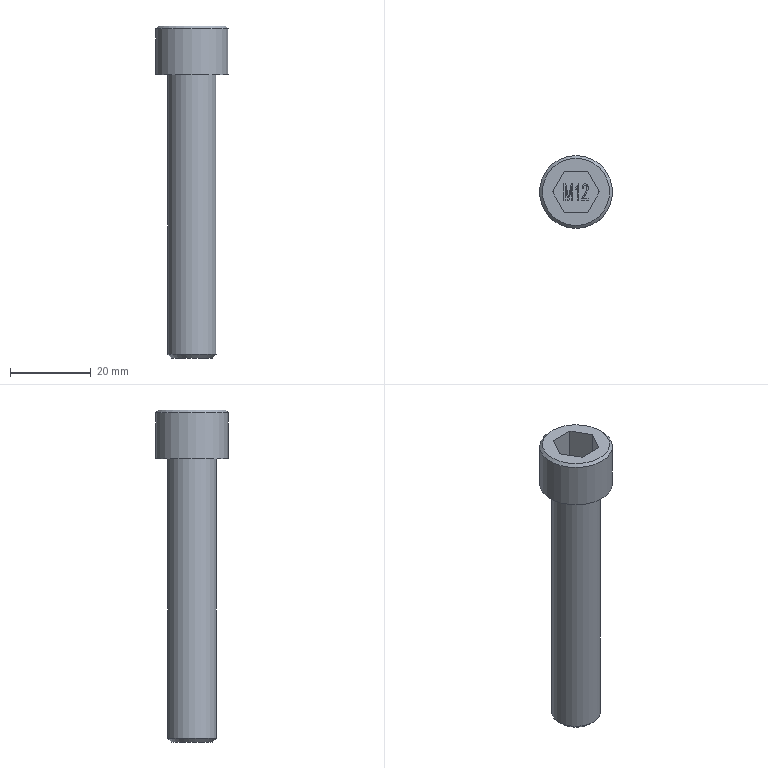Part | STEP file | EM11207000 | 1 solid | 43 faces | box 18 x 18 x 82 mm | volume 10251 mm3 | plane 33 | other 6 | cone 2 | cylinder 2 | commonest cylinder face diameters 12 x1 18 x1